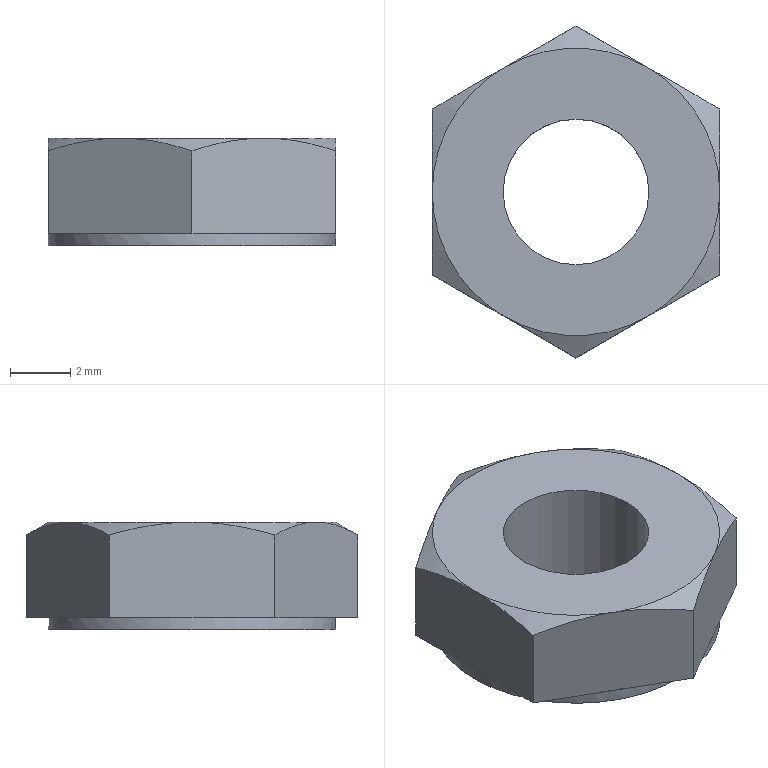Part | NX | features solid 2 | 1 solid | 22 faces | box 9.525 x 10.999 x 3.572 mm | volume 211.377 mm3 | plane 14 | cone 6 | cylinder 2 | commonest cylinder face diameters 4.826 x1 9.525 x1
STEP:
#1=CARTESIAN_POINT('',(2.381,4.124,3.572));
#2=VERTEX_POINT('',#1);
#3=CARTESIAN_POINT('',(0.,5.499,3.147));
#4=VERTEX_POINT('',#3);
#5=CARTESIAN_POINT('',(2.381,4.124,3.572));
#6=CARTESIAN_POINT('',(1.573,4.591,3.572));
#7=CARTESIAN_POINT('',(0.7771,5.051,3.406));
#8=CARTESIAN_POINT('',(0.,5.499,3.147));
#9=B_SPLINE_CURVE_WITH_KNOTS('',3,(#5,#6,#7,#8),.UNSPECIFIED.,.F.,.F.,(4,4),(0.002782,0.005554),.UNSPECIFIED.);
#10=EDGE_CURVE('',#2,#4,#9,.T.);
#11=ORIENTED_EDGE('',*,*,#10,.T.);
#12=CARTESIAN_POINT('',(-2.381,4.124,3.572));
#13=VERTEX_POINT('',#12);
#14=CARTESIAN_POINT('',(0.,5.499,3.147));
#15=CARTESIAN_POINT('',(-0.7791,5.049,3.406));
#16=CARTESIAN_POINT('',(-1.57,4.593,3.572));
#17=CARTESIAN_POINT('',(-2.381,4.124,3.572));
#18=B_SPLINE_CURVE_WITH_KNOTS('',3,(#14,#15,#16,#17),.UNSPECIFIED.,.F.,.F.,(4,4),(0.000000238,0.002782),.UNSPECIFIED.);
#19=EDGE_CURVE('',#4,#13,#18,.T.);
#20=ORIENTED_EDGE('',*,*,#19,.T.);
#21=CARTESIAN_POINT('',(0.,0.,3.572));
#22=DIRECTION('',(0.,0.,-1.));
#23=DIRECTION('',(-1.,0.,0.));
#24=AXIS2_PLACEMENT_3D('',#21,#22,#23);
#25=CIRCLE('',#24,4.763);
#26=EDGE_CURVE('',#13,#2,#25,.T.);
#27=ORIENTED_EDGE('',*,*,#26,.T.);
#28=EDGE_LOOP('',(#11,#20,#27));
#29=FACE_BOUND('',#28,.T.);
#30=CARTESIAN_POINT('',(0.,0.,3.572));
#31=DIRECTION('',(0.,0.,-1.));
#32=DIRECTION('',(-1.,0.,0.));
#33=AXIS2_PLACEMENT_3D('',#30,#31,#32);
#34=CONICAL_SURFACE('',#33,4.763,1.047);
#35=ADVANCED_FACE('',(#29),#34,.T.);
#36=CARTESIAN_POINT('',(-4.763,0.,3.572));
#37=VERTEX_POINT('',#36);
#38=CARTESIAN_POINT('',(0.,0.,3.572));
#39=DIRECTION('',(0.,0.,-1.));
#40=DIRECTION('',(-1.,0.,0.));
#41=AXIS2_PLACEMENT_3D('',#38,#39,#40);
#42=CIRCLE('',#41,4.763);
#43=EDGE_CURVE('',#37,#13,#42,.T.);
#44=ORIENTED_EDGE('',*,*,#43,.T.);
#45=CARTESIAN_POINT('',(-4.763,2.75,3.147));
#46=VERTEX_POINT('',#45);
#47=CARTESIAN_POINT('',(-2.381,4.124,3.572));
#48=CARTESIAN_POINT('',(-3.19,3.658,3.572));
#49=CARTESIAN_POINT('',(-3.985,3.198,3.406));
#50=CARTESIAN_POINT('',(-4.763,2.75,3.147));
#51=B_SPLINE_CURVE_WITH_KNOTS('',3,(#47,#48,#49,#50),.UNSPECIFIED.,.F.,.F.,(4,4),(0.002782,0.005554),.UNSPECIFIED.);
#52=EDGE_CURVE('',#13,#46,#51,.T.);
#53=ORIENTED_EDGE('',*,*,#52,.T.);
#54=CARTESIAN_POINT('',(-4.763,0.,3.572));
#55=CARTESIAN_POINT('',(-4.763,0.9308,3.572));
#56=CARTESIAN_POINT('',(-4.763,1.86,3.403));
#57=CARTESIAN_POINT('',(-4.763,2.75,3.147));
#58=B_SPLINE_CURVE_WITH_KNOTS('',3,(#54,#55,#56,#57),.UNSPECIFIED.,.F.,.F.,(4,4),(0.007836,0.01062),.UNSPECIFIED.);
#59=EDGE_CURVE('',#46,#37,#58,.F.);
#60=ORIENTED_EDGE('',*,*,#59,.T.);
#61=EDGE_LOOP('',(#44,#53,#60));
#62=FACE_BOUND('',#61,.T.);
#63=CARTESIAN_POINT('',(0.,0.,3.572));
#64=DIRECTION('',(0.,0.,-1.));
#65=DIRECTION('',(-1.,0.,0.));
#66=AXIS2_PLACEMENT_3D('',#63,#64,#65);
#67=CONICAL_SURFACE('',#66,4.763,1.047);
#68=ADVANCED_FACE('',(#62),#67,.T.);
#69=CARTESIAN_POINT('',(-2.381,-4.124,3.572));
#70=VERTEX_POINT('',#69);
#71=CARTESIAN_POINT('',(0.,0.,3.572));
#72=DIRECTION('',(0.,0.,-1.));
#73=DIRECTION('',(-1.,0.,0.));
#74=AXIS2_PLACEMENT_3D('',#71,#72,#73);
#75=CIRCLE('',#74,4.763);
#76=EDGE_CURVE('',#70,#37,#75,.T.);
#77=ORIENTED_EDGE('',*,*,#76,.T.);
#78=CARTESIAN_POINT('',(-4.763,-2.75,3.147));
#79=VERTEX_POINT('',#78);
#80=CARTESIAN_POINT('',(-4.763,-2.75,3.147));
#81=CARTESIAN_POINT('',(-4.763,-1.854,3.405));
#82=CARTESIAN_POINT('',(-4.763,-0.9302,3.572));
#83=CARTESIAN_POINT('',(-4.763,0.,3.572));
#84=B_SPLINE_CURVE_WITH_KNOTS('',3,(#80,#81,#82,#83),.UNSPECIFIED.,.F.,.F.,(4,4),(0.005053,0.007836),.UNSPECIFIED.);
#85=EDGE_CURVE('',#37,#79,#84,.F.);
#86=ORIENTED_EDGE('',*,*,#85,.T.);
#87=CARTESIAN_POINT('',(-4.763,-2.75,3.147));
#88=CARTESIAN_POINT('',(-3.983,-3.199,3.406));
#89=CARTESIAN_POINT('',(-3.193,-3.656,3.572));
#90=CARTESIAN_POINT('',(-2.381,-4.124,3.572));
#91=B_SPLINE_CURVE_WITH_KNOTS('',3,(#87,#88,#89,#90),.UNSPECIFIED.,.F.,.F.,(4,4),(0.000000238,0.002782),.UNSPECIFIED.);
#92=EDGE_CURVE('',#79,#70,#91,.T.);
#93=ORIENTED_EDGE('',*,*,#92,.T.);
#94=EDGE_LOOP('',(#77,#86,#93));
#95=FACE_BOUND('',#94,.T.);
#96=CARTESIAN_POINT('',(0.,0.,3.572));
#97=DIRECTION('',(0.,0.,-1.));
#98=DIRECTION('',(-1.,0.,0.));
#99=AXIS2_PLACEMENT_3D('',#96,#97,#98);
#100=CONICAL_SURFACE('',#99,4.763,1.047);
#101=ADVANCED_FACE('',(#95),#100,.T.);
#102=CARTESIAN_POINT('',(2.381,-4.124,3.572));
#103=VERTEX_POINT('',#102);
#104=CARTESIAN_POINT('',(0.,0.,3.572));
#105=DIRECTION('',(0.,0.,-1.));
#106=DIRECTION('',(-1.,0.,0.));
#107=AXIS2_PLACEMENT_3D('',#104,#105,#106);
#108=CIRCLE('',#107,4.763);
#109=EDGE_CURVE('',#103,#70,#108,.T.);
#110=ORIENTED_EDGE('',*,*,#109,.T.);
#111=CARTESIAN_POINT('',(0.,-5.499,3.147));
#112=VERTEX_POINT('',#111);
#113=CARTESIAN_POINT('',(-2.381,-4.124,3.572));
#114=CARTESIAN_POINT('',(-1.573,-4.591,3.572));
#115=CARTESIAN_POINT('',(-0.7771,-5.051,3.406));
#116=CARTESIAN_POINT('',(0.,-5.499,3.147));
#117=B_SPLINE_CURVE_WITH_KNOTS('',3,(#113,#114,#115,#116),.UNSPECIFIED.,.F.,.F.,(4,4),(0.002782,0.005554),.UNSPECIFIED.);
#118=EDGE_CURVE('',#70,#112,#117,.T.);
#119=ORIENTED_EDGE('',*,*,#118,.T.);
#120=CARTESIAN_POINT('',(0.,-5.499,3.147));
#121=CARTESIAN_POINT('',(0.7791,-5.049,3.406));
#122=CARTESIAN_POINT('',(1.57,-4.593,3.572));
#123=CARTESIAN_POINT('',(2.381,-4.124,3.572));
#124=B_SPLINE_CURVE_WITH_KNOTS('',3,(#120,#121,#122,#123),.UNSPECIFIED.,.F.,.F.,(4,4),(0.000000238,0.002782),.UNSPECIFIED.);
#125=EDGE_CURVE('',#112,#103,#124,.T.);
#126=ORIENTED_EDGE('',*,*,#125,.T.);
#127=EDGE_LOOP('',(#110,#119,#126));
#128=FACE_BOUND('',#127,.T.);
#129=CARTESIAN_POINT('',(0.,0.,3.572));
#130=DIRECTION('',(0.,0.,-1.));
#131=DIRECTION('',(-1.,0.,0.));
#132=AXIS2_PLACEMENT_3D('',#129,#130,#131);
#133=CONICAL_SURFACE('',#132,4.763,1.047);
#134=ADVANCED_FACE('',(#128),#133,.T.);
#135=CARTESIAN_POINT('',(4.763,0.,3.572));
#136=VERTEX_POINT('',#135);
#137=CARTESIAN_POINT('',(0.,0.,3.572));
#138=DIRECTION('',(0.,0.,-1.));
#139=DIRECTION('',(-1.,0.,0.));
#140=AXIS2_PLACEMENT_3D('',#137,#138,#139);
#141=CIRCLE('',#140,4.763);
#142=EDGE_CURVE('',#136,#103,#141,.T.);
#143=ORIENTED_EDGE('',*,*,#142,.T.);
#144=CARTESIAN_POINT('',(4.763,-2.75,3.147));
#145=VERTEX_POINT('',#144);
#146=CARTESIAN_POINT('',(2.381,-4.124,3.572));
#147=CARTESIAN_POINT('',(3.19,-3.658,3.572));
#148=CARTESIAN_POINT('',(3.985,-3.198,3.406));
#149=CARTESIAN_POINT('',(4.763,-2.75,3.147));
#150=B_SPLINE_CURVE_WITH_KNOTS('',3,(#146,#147,#148,#149),.UNSPECIFIED.,.F.,.F.,(4,4),(0.002782,0.005554),.UNSPECIFIED.);
#151=EDGE_CURVE('',#103,#145,#150,.T.);
#152=ORIENTED_EDGE('',*,*,#151,.T.);
#153=CARTESIAN_POINT('',(4.763,-2.75,3.147));
#154=CARTESIAN_POINT('',(4.763,-1.854,3.405));
#155=CARTESIAN_POINT('',(4.763,-0.9302,3.572));
#156=CARTESIAN_POINT('',(4.763,0.,3.572));
#157=B_SPLINE_CURVE_WITH_KNOTS('',3,(#153,#154,#155,#156),.UNSPECIFIED.,.F.,.F.,(4,4),(0.005053,0.007836),.UNSPECIFIED.);
#158=EDGE_CURVE('',#145,#136,#157,.T.);
#159=ORIENTED_EDGE('',*,*,#158,.T.);
#160=EDGE_LOOP('',(#143,#152,#159));
#161=FACE_BOUND('',#160,.T.);
#162=CARTESIAN_POINT('',(0.,0.,3.572));
#163=DIRECTION('',(0.,0.,-1.));
#164=DIRECTION('',(-1.,0.,0.));
#165=AXIS2_PLACEMENT_3D('',#162,#163,#164);
#166=CONICAL_SURFACE('',#165,4.763,1.047);
#167=ADVANCED_FACE('',(#161),#166,.T.);
#168=CARTESIAN_POINT('',(0.,0.,3.572));
#169=DIRECTION('',(0.,0.,-1.));
#170=DIRECTION('',(-1.,0.,0.));
#171=AXIS2_PLACEMENT_3D('',#168,#169,#170);
#172=CIRCLE('',#171,4.763);
#173=EDGE_CURVE('',#2,#136,#172,.T.);
#174=ORIENTED_EDGE('',*,*,#173,.T.);
#175=CARTESIAN_POINT('',(4.763,2.75,3.147));
#176=VERTEX_POINT('',#175);
#177=CARTESIAN_POINT('',(4.763,0.,3.572));
#178=CARTESIAN_POINT('',(4.763,0.9308,3.572));
#179=CARTESIAN_POINT('',(4.763,1.86,3.403));
#180=CARTESIAN_POINT('',(4.763,2.75,3.147));
#181=B_SPLINE_CURVE_WITH_KNOTS('',3,(#177,#178,#179,#180),.UNSPECIFIED.,.F.,.F.,(4,4),(0.007836,0.01062),.UNSPECIFIED.);
#182=EDGE_CURVE('',#136,#176,#181,.T.);
#183=ORIENTED_EDGE('',*,*,#182,.T.);
#184=CARTESIAN_POINT('',(4.763,2.75,3.147));
#185=CARTESIAN_POINT('',(3.983,3.199,3.406));
#186=CARTESIAN_POINT('',(3.193,3.656,3.572));
#187=CARTESIAN_POINT('',(2.381,4.124,3.572));
#188=B_SPLINE_CURVE_WITH_KNOTS('',3,(#184,#185,#186,#187),.UNSPECIFIED.,.F.,.F.,(4,4),(0.000000238,0.002782),.UNSPECIFIED.);
#189=EDGE_CURVE('',#176,#2,#188,.T.);
#190=ORIENTED_EDGE('',*,*,#189,.T.);
#191=EDGE_LOOP('',(#174,#183,#190));
#192=FACE_BOUND('',#191,.T.);
#193=CARTESIAN_POINT('',(0.,0.,3.572));
#194=DIRECTION('',(0.,0.,-1.));
#195=DIRECTION('',(-1.,0.,0.));
#196=AXIS2_PLACEMENT_3D('',#193,#194,#195);
#197=CONICAL_SURFACE('',#196,4.763,1.047);
#198=ADVANCED_FACE('',(#192),#197,.T.);
#199=CARTESIAN_POINT('',(2.381,-4.124,0.4064));
#200=VERTEX_POINT('',#199);
#201=CARTESIAN_POINT('',(0.,-5.499,0.4064));
#202=VERTEX_POINT('',#201);
#203=CARTESIAN_POINT('',(7.739,-1.031,0.4064));
#204=DIRECTION('',(-0.866,-0.5,0.));
#205=VECTOR('',#204,1000.);
#206=LINE('',#203,#205);
#207=EDGE_CURVE('',#200,#202,#206,.T.);
#208=ORIENTED_EDGE('',*,*,#207,.T.);
#209=CARTESIAN_POINT('',(-2.381,-4.124,0.4064));
#210=VERTEX_POINT('',#209);
#211=CARTESIAN_POINT('',(2.977,-7.218,0.4064));
#212=DIRECTION('',(-0.866,0.5,0.));
#213=VECTOR('',#212,1000.);
#214=LINE('',#211,#213);
#215=EDGE_CURVE('',#202,#210,#214,.T.);
#216=ORIENTED_EDGE('',*,*,#215,.T.);
#217=CARTESIAN_POINT('',(0.,0.,0.4064));
#218=DIRECTION('',(0.,0.,-1.));
#219=DIRECTION('',(-1.,0.,0.));
#220=AXIS2_PLACEMENT_3D('',#217,#218,#219);
#221=CIRCLE('',#220,4.763);
#222=EDGE_CURVE('',#200,#210,#221,.T.);
#223=ORIENTED_EDGE('',*,*,#222,.F.);
#224=EDGE_LOOP('',(#208,#216,#223));
#225=FACE_BOUND('',#224,.T.);
#226=CARTESIAN_POINT('',(7.144,0.,0.4064));
#227=DIRECTION('',(0.,0.,1.));
#228=DIRECTION('',(1.,0.,0.));
#229=AXIS2_PLACEMENT_3D('',#226,#227,#228);
#230=PLANE('',#229);
#231=ADVANCED_FACE('',(#225),#230,.F.);
#232=CARTESIAN_POINT('',(-4.763,0.,0.4064));
#233=VERTEX_POINT('',#232);
#234=CARTESIAN_POINT('',(0.,0.,0.4064));
#235=DIRECTION('',(0.,0.,-1.));
#236=DIRECTION('',(-1.,0.,0.));
#237=AXIS2_PLACEMENT_3D('',#234,#235,#236);
#238=CIRCLE('',#237,4.763);
#239=EDGE_CURVE('',#210,#233,#238,.T.);
#240=ORIENTED_EDGE('',*,*,#239,.F.);
#241=CARTESIAN_POINT('',(-4.763,-2.75,0.4064));
#242=VERTEX_POINT('',#241);
#243=CARTESIAN_POINT('',(2.977,-7.218,0.4064));
#244=DIRECTION('',(-0.866,0.5,0.));
#245=VECTOR('',#244,1000.);
#246=LINE('',#243,#245);
#247=EDGE_CURVE('',#210,#242,#246,.T.);
#248=ORIENTED_EDGE('',*,*,#247,.T.);
#249=CARTESIAN_POINT('',(-4.763,0.,0.4064));
#250=DIRECTION('',(0.,1.,0.));
#251=VECTOR('',#250,1000.);
#252=LINE('',#249,#251);
#253=EDGE_CURVE('',#242,#233,#252,.T.);
#254=ORIENTED_EDGE('',*,*,#253,.T.);
#255=EDGE_LOOP('',(#240,#248,#254));
#256=FACE_BOUND('',#255,.T.);
#257=CARTESIAN_POINT('',(7.144,0.,0.4064));
#258=DIRECTION('',(0.,0.,1.));
#259=DIRECTION('',(1.,0.,0.));
#260=AXIS2_PLACEMENT_3D('',#257,#258,#259);
#261=PLANE('',#260);
#262=ADVANCED_FACE('',(#256),#261,.F.);
#263=CARTESIAN_POINT('',(-2.381,4.124,0.4064));
#264=VERTEX_POINT('',#263);
#265=CARTESIAN_POINT('',(0.,0.,0.4064));
#266=DIRECTION('',(0.,0.,-1.));
#267=DIRECTION('',(-1.,0.,0.));
#268=AXIS2_PLACEMENT_3D('',#265,#266,#267);
#269=CIRCLE('',#268,4.763);
#270=EDGE_CURVE('',#233,#264,#269,.T.);
#271=ORIENTED_EDGE('',*,*,#270,.F.);
#272=CARTESIAN_POINT('',(-4.763,2.75,0.4064));
#273=VERTEX_POINT('',#272);
#274=CARTESIAN_POINT('',(-4.763,0.,0.4064));
#275=DIRECTION('',(0.,1.,0.));
#276=VECTOR('',#275,1000.);
#277=LINE('',#274,#276);
#278=EDGE_CURVE('',#233,#273,#277,.T.);
#279=ORIENTED_EDGE('',*,*,#278,.T.);
#280=CARTESIAN_POINT('',(2.977,7.218,0.4064));
#281=DIRECTION('',(0.866,0.5,0.));
#282=VECTOR('',#281,1000.);
#283=LINE('',#280,#282);
#284=EDGE_CURVE('',#273,#264,#283,.T.);
#285=ORIENTED_EDGE('',*,*,#284,.T.);
#286=EDGE_LOOP('',(#271,#279,#285));
#287=FACE_BOUND('',#286,.T.);
#288=CARTESIAN_POINT('',(7.144,0.,0.4064));
#289=DIRECTION('',(0.,0.,1.));
#290=DIRECTION('',(1.,0.,0.));
#291=AXIS2_PLACEMENT_3D('',#288,#289,#290);
#292=PLANE('',#291);
#293=ADVANCED_FACE('',(#287),#292,.F.);
#294=CARTESIAN_POINT('',(4.763,0.,0.4064));
#295=VERTEX_POINT('',#294);
#296=CARTESIAN_POINT('',(4.763,-2.75,0.4064));
#297=VERTEX_POINT('',#296);
#298=CARTESIAN_POINT('',(4.763,0.,0.4064));
#299=DIRECTION('',(0.,-1.,0.));
#300=VECTOR('',#299,1000.);
#301=LINE('',#298,#300);
#302=EDGE_CURVE('',#295,#297,#301,.T.);
#303=ORIENTED_EDGE('',*,*,#302,.T.);
#304=CARTESIAN_POINT('',(7.739,-1.031,0.4064));
#305=DIRECTION('',(-0.866,-0.5,0.));
#306=VECTOR('',#305,1000.);
#307=LINE('',#304,#306);
#308=EDGE_CURVE('',#297,#200,#307,.T.);
#309=ORIENTED_EDGE('',*,*,#308,.T.);
#310=CARTESIAN_POINT('',(0.,0.,0.4064));
#311=DIRECTION('',(0.,0.,-1.));
#312=DIRECTION('',(-1.,0.,0.));
#313=AXIS2_PLACEMENT_3D('',#310,#311,#312);
#314=CIRCLE('',#313,4.763);
#315=EDGE_CURVE('',#295,#200,#314,.T.);
#316=ORIENTED_EDGE('',*,*,#315,.F.);
#317=EDGE_LOOP('',(#303,#309,#316));
#318=FACE_BOUND('',#317,.T.);
#319=CARTESIAN_POINT('',(7.144,0.,0.4064));
#320=DIRECTION('',(0.,0.,1.));
#321=DIRECTION('',(1.,0.,0.));
#322=AXIS2_PLACEMENT_3D('',#319,#320,#321);
#323=PLANE('',#322);
#324=ADVANCED_FACE('',(#318),#323,.F.);
#325=CARTESIAN_POINT('',(2.381,4.124,0.4064));
#326=VERTEX_POINT('',#325);
#327=CARTESIAN_POINT('',(0.,0.,0.4064));
#328=DIRECTION('',(0.,0.,-1.));
#329=DIRECTION('',(-1.,0.,0.));
#330=AXIS2_PLACEMENT_3D('',#327,#328,#329);
#331=CIRCLE('',#330,4.763);
#332=EDGE_CURVE('',#264,#326,#331,.T.);
#333=ORIENTED_EDGE('',*,*,#332,.F.);
#334=CARTESIAN_POINT('',(0.,5.499,0.4064));
#335=VERTEX_POINT('',#334);
#336=CARTESIAN_POINT('',(2.977,7.218,0.4064));
#337=DIRECTION('',(0.866,0.5,0.));
#338=VECTOR('',#337,1000.);
#339=LINE('',#336,#338);
#340=EDGE_CURVE('',#264,#335,#339,.T.);
#341=ORIENTED_EDGE('',*,*,#340,.T.);
#342=CARTESIAN_POINT('',(7.739,1.031,0.4064));
#343=DIRECTION('',(0.866,-0.5,0.));
#344=VECTOR('',#343,1000.);
#345=LINE('',#342,#344);
#346=EDGE_CURVE('',#335,#326,#345,.T.);
#347=ORIENTED_EDGE('',*,*,#346,.T.);
#348=EDGE_LOOP('',(#333,#341,#347));
#349=FACE_BOUND('',#348,.T.);
#350=CARTESIAN_POINT('',(7.144,0.,0.4064));
#351=DIRECTION('',(0.,0.,1.));
#352=DIRECTION('',(1.,0.,0.));
#353=AXIS2_PLACEMENT_3D('',#350,#351,#352);
#354=PLANE('',#353);
#355=ADVANCED_FACE('',(#349),#354,.F.);
#356=CARTESIAN_POINT('',(4.763,2.75,0.4064));
#357=VERTEX_POINT('',#356);
#358=CARTESIAN_POINT('',(7.739,1.031,0.4064));
#359=DIRECTION('',(0.866,-0.5,0.));
#360=VECTOR('',#359,1000.);
#361=LINE('',#358,#360);
#362=EDGE_CURVE('',#326,#357,#361,.T.);
#363=ORIENTED_EDGE('',*,*,#362,.T.);
#364=CARTESIAN_POINT('',(4.763,0.,0.4064));
#365=DIRECTION('',(0.,-1.,0.));
#366=VECTOR('',#365,1000.);
#367=LINE('',#364,#366);
#368=EDGE_CURVE('',#357,#295,#367,.T.);
#369=ORIENTED_EDGE('',*,*,#368,.T.);
#370=CARTESIAN_POINT('',(0.,0.,0.4064));
#371=DIRECTION('',(0.,0.,-1.));
#372=DIRECTION('',(-1.,0.,0.));
#373=AXIS2_PLACEMENT_3D('',#370,#371,#372);
#374=CIRCLE('',#373,4.763);
#375=EDGE_CURVE('',#326,#295,#374,.T.);
#376=ORIENTED_EDGE('',*,*,#375,.F.);
#377=EDGE_LOOP('',(#363,#369,#376));
#378=FACE_BOUND('',#377,.T.);
#379=CARTESIAN_POINT('',(7.144,0.,0.4064));
#380=DIRECTION('',(0.,0.,1.));
#381=DIRECTION('',(1.,0.,0.));
#382=AXIS2_PLACEMENT_3D('',#379,#380,#381);
#383=PLANE('',#382);
#384=ADVANCED_FACE('',(#378),#383,.F.);
#385=ORIENTED_EDGE('',*,*,#43,.F.);
#386=ORIENTED_EDGE('',*,*,#76,.F.);
#387=ORIENTED_EDGE('',*,*,#109,.F.);
#388=ORIENTED_EDGE('',*,*,#142,.F.);
#389=ORIENTED_EDGE('',*,*,#173,.F.);
#390=ORIENTED_EDGE('',*,*,#26,.F.);
#391=EDGE_LOOP('',(#385,#386,#387,#388,#389,#390));
#392=FACE_BOUND('',#391,.T.);
#393=CARTESIAN_POINT('',(-2.413,0.,3.572));
#394=VERTEX_POINT('',#393);
#395=CARTESIAN_POINT('',(0.,0.,3.572));
#396=DIRECTION('',(0.,0.,-1.));
#397=DIRECTION('',(-1.,0.,0.));
#398=AXIS2_PLACEMENT_3D('',#395,#396,#397);
#399=CIRCLE('',#398,2.413);
#400=EDGE_CURVE('',#394,#394,#399,.T.);
#401=ORIENTED_EDGE('',*,*,#400,.T.);
#402=EDGE_LOOP('',(#401));
#403=FACE_BOUND('',#402,.T.);
#404=CARTESIAN_POINT('',(2.413,0.,3.572));
#405=DIRECTION('',(0.,0.,-1.));
#406=DIRECTION('',(-1.,0.,0.));
#407=AXIS2_PLACEMENT_3D('',#404,#405,#406);
#408=PLANE('',#407);
#409=ADVANCED_FACE('',(#392,#403),#408,.F.);
#410=CARTESIAN_POINT('',(-4.763,0.,0.));
#411=VERTEX_POINT('',#410);
#412=CARTESIAN_POINT('',(0.,0.,0.));
#413=DIRECTION('',(0.,0.,-1.));
#414=DIRECTION('',(-1.,0.,0.));
#415=AXIS2_PLACEMENT_3D('',#412,#413,#414);
#416=CIRCLE('',#415,4.763);
#417=EDGE_CURVE('',#411,#411,#416,.T.);
#418=ORIENTED_EDGE('',*,*,#417,.F.);
#419=EDGE_LOOP('',(#418));
#420=FACE_BOUND('',#419,.T.);
#421=ORIENTED_EDGE('',*,*,#270,.T.);
#422=ORIENTED_EDGE('',*,*,#332,.T.);
#423=ORIENTED_EDGE('',*,*,#375,.T.);
#424=ORIENTED_EDGE('',*,*,#315,.T.);
#425=ORIENTED_EDGE('',*,*,#222,.T.);
#426=ORIENTED_EDGE('',*,*,#239,.T.);
#427=EDGE_LOOP('',(#421,#422,#423,#424,#425,#426));
#428=FACE_BOUND('',#427,.T.);
#429=CARTESIAN_POINT('',(0.,0.,0.));
#430=DIRECTION('',(0.,0.,-1.));
#431=DIRECTION('',(-1.,0.,0.));
#432=AXIS2_PLACEMENT_3D('',#429,#430,#431);
#433=CYLINDRICAL_SURFACE('',#432,4.763);
#434=ADVANCED_FACE('',(#420,#428),#433,.T.);
#435=CARTESIAN_POINT('',(-2.413,0.,0.));
#436=VERTEX_POINT('',#435);
#437=CARTESIAN_POINT('',(0.,0.,0.));
#438=DIRECTION('',(0.,0.,-1.));
#439=DIRECTION('',(-1.,0.,0.));
#440=AXIS2_PLACEMENT_3D('',#437,#438,#439);
#441=CIRCLE('',#440,2.413);
#442=EDGE_CURVE('',#436,#436,#441,.T.);
#443=ORIENTED_EDGE('',*,*,#442,.F.);
#444=EDGE_LOOP('',(#443));
#445=FACE_BOUND('',#444,.T.);
#446=ORIENTED_EDGE('',*,*,#417,.T.);
#447=EDGE_LOOP('',(#446));
#448=FACE_BOUND('',#447,.T.);
#449=CARTESIAN_POINT('',(4.763,0.,0.));
#450=DIRECTION('',(0.,0.,1.));
#451=DIRECTION('',(1.,0.,0.));
#452=AXIS2_PLACEMENT_3D('',#449,#450,#451);
#453=PLANE('',#452);
#454=ADVANCED_FACE('',(#445,#448),#453,.F.);
#455=ORIENTED_EDGE('',*,*,#400,.F.);
#456=EDGE_LOOP('',(#455));
#457=FACE_BOUND('',#456,.T.);
#458=ORIENTED_EDGE('',*,*,#442,.T.);
#459=EDGE_LOOP('',(#458));
#460=FACE_BOUND('',#459,.T.);
#461=CARTESIAN_POINT('',(0.,0.,0.));
#462=DIRECTION('',(0.,0.,-1.));
#463=DIRECTION('',(-1.,0.,0.));
#464=AXIS2_PLACEMENT_3D('',#461,#462,#463);
#465=CYLINDRICAL_SURFACE('',#464,2.413);
#466=ADVANCED_FACE('',(#457,#460),#465,.F.);
#467=ORIENTED_EDGE('',*,*,#19,.F.);
#468=CARTESIAN_POINT('',(0.,5.499,3.929));
#469=DIRECTION('',(0.,0.,-1.));
#470=VECTOR('',#469,1000.);
#471=LINE('',#468,#470);
#472=EDGE_CURVE('',#4,#335,#471,.T.);
#473=ORIENTED_EDGE('',*,*,#472,.T.);
#474=ORIENTED_EDGE('',*,*,#340,.F.);
#475=ORIENTED_EDGE('',*,*,#284,.F.);
#476=CARTESIAN_POINT('',(-4.763,2.75,3.929));
#477=DIRECTION('',(0.,0.,-1.));
#478=VECTOR('',#477,1000.);
#479=LINE('',#476,#478);
#480=EDGE_CURVE('',#46,#273,#479,.T.);
#481=ORIENTED_EDGE('',*,*,#480,.F.);
#482=ORIENTED_EDGE('',*,*,#52,.F.);
#483=EDGE_LOOP('',(#467,#473,#474,#475,#481,#482));
#484=FACE_BOUND('',#483,.T.);
#485=CARTESIAN_POINT('',(0.,5.499,3.929));
#486=DIRECTION('',(0.5,-0.866,0.));
#487=DIRECTION('',(0.866,0.5,0.));
#488=AXIS2_PLACEMENT_3D('',#485,#486,#487);
#489=PLANE('',#488);
#490=ADVANCED_FACE('',(#484),#489,.F.);
#491=ORIENTED_EDGE('',*,*,#59,.F.);
#492=ORIENTED_EDGE('',*,*,#480,.T.);
#493=ORIENTED_EDGE('',*,*,#278,.F.);
#494=ORIENTED_EDGE('',*,*,#253,.F.);
#495=CARTESIAN_POINT('',(-4.763,-2.75,3.929));
#496=DIRECTION('',(0.,0.,-1.));
#497=VECTOR('',#496,1000.);
#498=LINE('',#495,#497);
#499=EDGE_CURVE('',#79,#242,#498,.T.);
#500=ORIENTED_EDGE('',*,*,#499,.F.);
#501=ORIENTED_EDGE('',*,*,#85,.F.);
#502=EDGE_LOOP('',(#491,#492,#493,#494,#500,#501));
#503=FACE_BOUND('',#502,.T.);
#504=CARTESIAN_POINT('',(-4.763,2.75,3.929));
#505=DIRECTION('',(1.,0.,0.));
#506=DIRECTION('',(0.,1.,0.));
#507=AXIS2_PLACEMENT_3D('',#504,#505,#506);
#508=PLANE('',#507);
#509=ADVANCED_FACE('',(#503),#508,.F.);
#510=ORIENTED_EDGE('',*,*,#92,.F.);
#511=ORIENTED_EDGE('',*,*,#499,.T.);
#512=ORIENTED_EDGE('',*,*,#247,.F.);
#513=ORIENTED_EDGE('',*,*,#215,.F.);
#514=CARTESIAN_POINT('',(0.,-5.499,3.929));
#515=DIRECTION('',(0.,0.,-1.));
#516=VECTOR('',#515,1000.);
#517=LINE('',#514,#516);
#518=EDGE_CURVE('',#112,#202,#517,.T.);
#519=ORIENTED_EDGE('',*,*,#518,.F.);
#520=ORIENTED_EDGE('',*,*,#118,.F.);
#521=EDGE_LOOP('',(#510,#511,#512,#513,#519,#520));
#522=FACE_BOUND('',#521,.T.);
#523=CARTESIAN_POINT('',(-4.763,-2.75,3.929));
#524=DIRECTION('',(0.5,0.866,0.));
#525=DIRECTION('',(-0.866,0.5,0.));
#526=AXIS2_PLACEMENT_3D('',#523,#524,#525);
#527=PLANE('',#526);
#528=ADVANCED_FACE('',(#522),#527,.F.);
#529=ORIENTED_EDGE('',*,*,#125,.F.);
#530=ORIENTED_EDGE('',*,*,#518,.T.);
#531=ORIENTED_EDGE('',*,*,#207,.F.);
#532=ORIENTED_EDGE('',*,*,#308,.F.);
#533=CARTESIAN_POINT('',(4.763,-2.75,3.929));
#534=DIRECTION('',(0.,0.,-1.));
#535=VECTOR('',#534,1000.);
#536=LINE('',#533,#535);
#537=EDGE_CURVE('',#145,#297,#536,.T.);
#538=ORIENTED_EDGE('',*,*,#537,.F.);
#539=ORIENTED_EDGE('',*,*,#151,.F.);
#540=EDGE_LOOP('',(#529,#530,#531,#532,#538,#539));
#541=FACE_BOUND('',#540,.T.);
#542=CARTESIAN_POINT('',(0.,-5.499,3.929));
#543=DIRECTION('',(-0.5,0.866,0.));
#544=DIRECTION('',(-0.866,-0.5,0.));
#545=AXIS2_PLACEMENT_3D('',#542,#543,#544);
#546=PLANE('',#545);
#547=ADVANCED_FACE('',(#541),#546,.F.);
#548=ORIENTED_EDGE('',*,*,#158,.F.);
#549=ORIENTED_EDGE('',*,*,#537,.T.);
#550=ORIENTED_EDGE('',*,*,#302,.F.);
#551=ORIENTED_EDGE('',*,*,#368,.F.);
#552=CARTESIAN_POINT('',(4.763,2.75,3.929));
#553=DIRECTION('',(0.,0.,-1.));
#554=VECTOR('',#553,1000.);
#555=LINE('',#552,#554);
#556=EDGE_CURVE('',#176,#357,#555,.T.);
#557=ORIENTED_EDGE('',*,*,#556,.F.);
#558=ORIENTED_EDGE('',*,*,#182,.F.);
#559=EDGE_LOOP('',(#548,#549,#550,#551,#557,#558));
#560=FACE_BOUND('',#559,.T.);
#561=CARTESIAN_POINT('',(4.763,-2.75,3.929));
#562=DIRECTION('',(-1.,0.,0.));
#563=DIRECTION('',(0.,0.,1.));
#564=AXIS2_PLACEMENT_3D('',#561,#562,#563);
#565=PLANE('',#564);
#566=ADVANCED_FACE('',(#560),#565,.F.);
#567=ORIENTED_EDGE('',*,*,#189,.F.);
#568=ORIENTED_EDGE('',*,*,#556,.T.);
#569=ORIENTED_EDGE('',*,*,#362,.F.);
#570=ORIENTED_EDGE('',*,*,#346,.F.);
#571=ORIENTED_EDGE('',*,*,#472,.F.);
#572=ORIENTED_EDGE('',*,*,#10,.F.);
#573=EDGE_LOOP('',(#567,#568,#569,#570,#571,#572));
#574=FACE_BOUND('',#573,.T.);
#575=CARTESIAN_POINT('',(4.763,2.75,3.929));
#576=DIRECTION('',(-0.5,-0.866,0.));
#577=DIRECTION('',(0.866,-0.5,0.));
#578=AXIS2_PLACEMENT_3D('',#575,#576,#577);
#579=PLANE('',#578);
#580=ADVANCED_FACE('',(#574),#579,.F.);
#581=CLOSED_SHELL('',(#35,#68,#101,#134,#167,#198,#231,#262,#293,#324,#355,#384,#409,#434,#454,#466,#490,#509,#528,#547,#566,#580));
#582=MANIFOLD_SOLID_BREP('',#581);
#583=(LENGTH_UNIT()NAMED_UNIT(*)SI_UNIT(.MILLI.,.METRE.));
#584=UNCERTAINTY_MEASURE_WITH_UNIT(LENGTH_MEASURE(0.0508),#583,'','');
#585=(NAMED_UNIT(*)PLANE_ANGLE_UNIT()SI_UNIT($,.RADIAN.));
#586=(NAMED_UNIT(*)SI_UNIT($,.STERADIAN.)SOLID_ANGLE_UNIT());
#587=(GEOMETRIC_REPRESENTATION_CONTEXT(3)GLOBAL_UNCERTAINTY_ASSIGNED_CONTEXT((#584))GLOBAL_UNIT_ASSIGNED_CONTEXT((#583,#585,#586))REPRESENTATION_CONTEXT('',''));
#588=ADVANCED_BREP_SHAPE_REPRESENTATION('',(#582),#587);